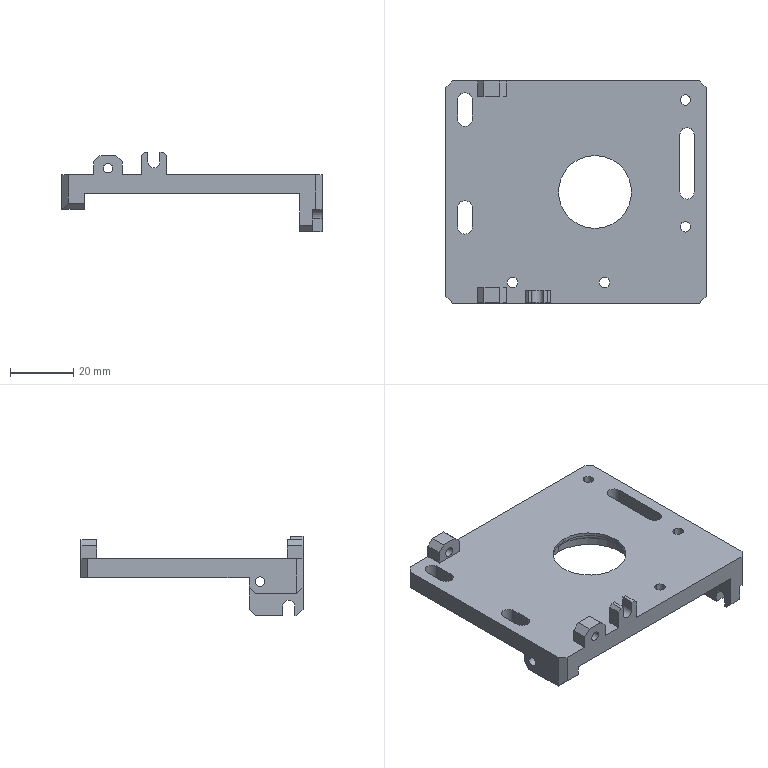NC program | NX | posted with a generic post | part box 82 x 70 x 25 mm
Lines 1 to 1705 of 7981:
N10 G17 G21 G94 G90
(FLOOR_WALL , TOOL : D20R0.8)
N12 T01 M6
N14 G54
N16 G17 G0 G90 X-56. Y36.999 S7500 M3
N18 G43 Z30. H1
N20 Z3.
N22 G94 G1 Z0. F1350.
N24 X-53.
N26 X53.
N28 Y27.479
N30 X-53.
N32 Y17.959
N34 X53.
N36 Y8.439
N38 X-53.
N40 Y-1.08
N42 X53.
N44 Y-10.6
N46 X-53.
N48 Y-20.12
N50 X53.
N52 Y-29.64
N54 X-53.
N56 X-56.
N58 Z3.
N60 G0 Z30.
N62 M5
(ZLEVEL_PROFILE_1 , TOOL : D6)
N64 T06 M6
N66 G54
N68 G17 G0 G90 X-34.289 Y38.1 S9500 M3
N70 G43 Z30. H6
N72 Z1.5
N74 G94 G1 X0. Z-0.297 F1000.
N76 X39. F3000.
N78 G2 X41.192 Y37.192 R3.1
N80 G1 X43.192 Y35.192
N82 G2 X44.1 Y33. R3.1
N84 G1 Y-33.
N86 G2 X43.192 Y-35.192 R3.1
N88 G1 X41.192 Y-37.192
N90 G2 X39. Y-38.1 R3.1
N92 G1 X-39.
N94 G2 X-41.192 Y-37.192 R3.1
N96 G1 X-43.192 Y-35.192
N98 G2 X-44.1 Y-33. R3.1
N100 G1 Y33.
N102 G2 X-43.192 Y35.192 R3.1
N104 G1 X-41.192 Y37.192
N106 G2 X-39. Y38.1 R3.1
N108 G1 X0.
N110 X17.016 Z-0.594
N112 X39.
N114 G2 X41.192 Y37.192 R3.1
N116 G1 X43.192 Y35.192
N118 G2 X44.1 Y33. R3.1
N120 G1 Y-33.
N122 G2 X43.192 Y-35.192 R3.1
N124 G1 X41.192 Y-37.192
N126 G2 X39. Y-38.1 R3.1
N128 G1 X-39.
N130 G2 X-41.192 Y-37.192 R3.1
N132 G1 X-43.192 Y-35.192
N134 G2 X-44.1 Y-33. R3.1
N136 G1 Y33.
N138 G2 X-43.192 Y35.192 R3.1
N140 G1 X-41.192 Y37.192
N142 G2 X-39. Y38.1 R3.1
N144 G1 X0.
N146 X17.016 Z-0.891
N148 X39.
N150 G2 X41.192 Y37.192 R3.1
N152 G1 X43.192 Y35.192
N154 G2 X44.1 Y33. R3.1
N156 G1 Y-33.
N158 G2 X43.192 Y-35.192 R3.1
N160 G1 X41.192 Y-37.192
N162 G2 X39. Y-38.1 R3.1
N164 G1 X-39.
N166 G2 X-41.192 Y-37.192 R3.1
N168 G1 X-43.192 Y-35.192
N170 G2 X-44.1 Y-33. R3.1
N172 G1 Y33.
N174 G2 X-43.192 Y35.192 R3.1
N176 G1 X-41.192 Y37.192
N178 G2 X-39. Y38.1 R3.1
N180 G1 X0.
N182 X17.016 Z-1.188
N184 X39.
N186 G2 X41.192 Y37.192 R3.1
N188 G1 X43.192 Y35.192
N190 G2 X44.1 Y33. R3.1
N192 G1 Y-33.
N194 G2 X43.192 Y-35.192 R3.1
N196 G1 X41.192 Y-37.192
N198 G2 X39. Y-38.1 R3.1
N200 G1 X-39.
N202 G2 X-41.192 Y-37.192 R3.1
N204 G1 X-43.192 Y-35.192
N206 G2 X-44.1 Y-33. R3.1
N208 G1 Y33.
N210 G2 X-43.192 Y35.192 R3.1
N212 G1 X-41.192 Y37.192
N214 G2 X-39. Y38.1 R3.1
N216 G1 X0.
N218 X17.016 Z-1.485
N220 X39.
N222 G2 X41.192 Y37.192 R3.1
N224 G1 X43.192 Y35.192
N226 G2 X44.1 Y33. R3.1
N228 G1 Y-33.
N230 G2 X43.192 Y-35.192 R3.1
N232 G1 X41.192 Y-37.192
N234 G2 X39. Y-38.1 R3.1
N236 G1 X-39.
N238 G2 X-41.192 Y-37.192 R3.1
N240 G1 X-43.192 Y-35.192
N242 G2 X-44.1 Y-33. R3.1
N244 G1 Y33.
N246 G2 X-43.192 Y35.192 R3.1
N248 G1 X-41.192 Y37.192
N250 G2 X-39. Y38.1 R3.1
N252 G1 X0.
N254 X17.016 Z-1.782
N256 X39.
N258 G2 X41.192 Y37.192 R3.1
N260 G1 X43.192 Y35.192
N262 G2 X44.1 Y33. R3.1
N264 G1 Y-33.
N266 G2 X43.192 Y-35.192 R3.1
N268 G1 X41.192 Y-37.192
N270 G2 X39. Y-38.1 R3.1
N272 G1 X-39.
N274 G2 X-41.192 Y-37.192 R3.1
N276 G1 X-43.192 Y-35.192
N278 G2 X-44.1 Y-33. R3.1
N280 G1 Y33.
N282 G2 X-43.192 Y35.192 R3.1
N284 G1 X-41.192 Y37.192
N286 G2 X-39. Y38.1 R3.1
N288 G1 X0.
N290 X17.016 Z-2.079
N292 X39.
N294 G2 X41.192 Y37.192 R3.1
N296 G1 X43.192 Y35.192
N298 G2 X44.1 Y33. R3.1
N300 G1 Y-33.
N302 G2 X43.192 Y-35.192 R3.1
N304 G1 X41.192 Y-37.192
N306 G2 X39. Y-38.1 R3.1
N308 G1 X-39.
N310 G2 X-41.192 Y-37.192 R3.1
N312 G1 X-43.192 Y-35.192
N314 G2 X-44.1 Y-33. R3.1
N316 G1 Y33.
N318 G2 X-43.192 Y35.192 R3.1
N320 G1 X-41.192 Y37.192
N322 G2 X-39. Y38.1 R3.1
N324 G1 X0.
N326 X17.016 Z-2.376
N328 X39.
N330 G2 X41.192 Y37.192 R3.1
N332 G1 X43.192 Y35.192
N334 G2 X44.1 Y33. R3.1
N336 G1 Y-33.
N338 G2 X43.192 Y-35.192 R3.1
N340 G1 X41.192 Y-37.192
N342 G2 X39. Y-38.1 R3.1
N344 G1 X-39.
N346 G2 X-41.192 Y-37.192 R3.1
N348 G1 X-43.192 Y-35.192
N350 G2 X-44.1 Y-33. R3.1
N352 G1 Y33.
N354 G2 X-43.192 Y35.192 R3.1
N356 G1 X-41.192 Y37.192
N358 G2 X-39. Y38.1 R3.1
N360 G1 X0.
N362 X17.016 Z-2.673
N364 X39.
N366 G2 X41.192 Y37.192 R3.1
N368 G1 X43.192 Y35.192
N370 G2 X44.1 Y33. R3.1
N372 G1 Y-33.
N374 G2 X43.192 Y-35.192 R3.1
N376 G1 X41.192 Y-37.192
N378 G2 X39. Y-38.1 R3.1
N380 G1 X-39.
N382 G2 X-41.192 Y-37.192 R3.1
N384 G1 X-43.192 Y-35.192
N386 G2 X-44.1 Y-33. R3.1
N388 G1 Y33.
N390 G2 X-43.192 Y35.192 R3.1
N392 G1 X-41.192 Y37.192
N394 G2 X-39. Y38.1 R3.1
N396 G1 X0.
N398 X17.016 Z-2.97
N400 X39.
N402 G2 X41.192 Y37.192 R3.1
N404 G1 X43.192 Y35.192
N406 G2 X44.1 Y33. R3.1
N408 G1 Y-33.
N410 G2 X43.192 Y-35.192 R3.1
N412 G1 X41.192 Y-37.192
N414 G2 X39. Y-38.1 R3.1
N416 G1 X-39.
N418 G2 X-41.192 Y-37.192 R3.1
N420 G1 X-43.192 Y-35.192
N422 G2 X-44.1 Y-33. R3.1
N424 G1 Y33.
N426 G2 X-43.192 Y35.192 R3.1
N428 G1 X-41.192 Y37.192
N430 G2 X-39. Y38.1 R3.1
N432 G1 X0.
N434 X17.016 Z-3.267
N436 X39.
N438 G2 X41.192 Y37.192 R3.1
N440 G1 X43.192 Y35.192
N442 G2 X44.1 Y33. R3.1
N444 G1 Y-33.
N446 G2 X43.192 Y-35.192 R3.1
N448 G1 X41.192 Y-37.192
N450 G2 X39. Y-38.1 R3.1
N452 G1 X-39.
N454 G2 X-41.192 Y-37.192 R3.1
N456 G1 X-43.192 Y-35.192
N458 G2 X-44.1 Y-33. R3.1
N460 G1 Y33.
N462 G2 X-43.192 Y35.192 R3.1
N464 G1 X-41.192 Y37.192
N466 G2 X-39. Y38.1 R3.1
N468 G1 X0.
N470 X17.016 Z-3.564
N472 X39.
N474 G2 X41.192 Y37.192 R3.1
N476 G1 X43.192 Y35.192
N478 G2 X44.1 Y33. R3.1
N480 G1 Y-33.
N482 G2 X43.192 Y-35.192 R3.1
N484 G1 X41.192 Y-37.192
N486 G2 X39. Y-38.1 R3.1
N488 G1 X-39.
N490 G2 X-41.192 Y-37.192 R3.1
N492 G1 X-43.192 Y-35.192
N494 G2 X-44.1 Y-33. R3.1
N496 G1 Y33.
N498 G2 X-43.192 Y35.192 R3.1
N500 G1 X-41.192 Y37.192
N502 G2 X-39. Y38.1 R3.1
N504 G1 X0.
N506 X17.016 Z-3.861
N508 X39.
N510 G2 X41.192 Y37.192 R3.1
N512 G1 X43.192 Y35.192
N514 G2 X44.1 Y33. R3.1
N516 G1 Y-33.
N518 G2 X43.192 Y-35.192 R3.1
N520 G1 X41.192 Y-37.192
N522 G2 X39. Y-38.1 R3.1
N524 G1 X-39.
N526 G2 X-41.192 Y-37.192 R3.1
N528 G1 X-43.192 Y-35.192
N530 G2 X-44.1 Y-33. R3.1
N532 G1 Y33.
N534 G2 X-43.192 Y35.192 R3.1
N536 G1 X-41.192 Y37.192
N538 G2 X-39. Y38.1 R3.1
N540 G1 X0.
N542 X17.016 Z-4.158
N544 X39.
N546 G2 X41.192 Y37.192 R3.1
N548 G1 X43.192 Y35.192
N550 G2 X44.1 Y33. R3.1
N552 G1 Y-33.
N554 G2 X43.192 Y-35.192 R3.1
N556 G1 X41.192 Y-37.192
N558 G2 X39. Y-38.1 R3.1
N560 G1 X-39.
N562 G2 X-41.192 Y-37.192 R3.1
N564 G1 X-43.192 Y-35.192
N566 G2 X-44.1 Y-33. R3.1
N568 G1 Y33.
N570 G2 X-43.192 Y35.192 R3.1
N572 G1 X-41.192 Y37.192
N574 G2 X-39. Y38.1 R3.1
N576 G1 X0.
N578 X17.016 Z-4.455
N580 X39.
N582 G2 X41.192 Y37.192 R3.1
N584 G1 X43.192 Y35.192
N586 G2 X44.1 Y33. R3.1
N588 G1 Y-33.
N590 G2 X43.192 Y-35.192 R3.1
N592 G1 X41.192 Y-37.192
N594 G2 X39. Y-38.1 R3.1
N596 G1 X-39.
N598 G2 X-41.192 Y-37.192 R3.1
N600 G1 X-43.192 Y-35.192
N602 G2 X-44.1 Y-33. R3.1
N604 G1 Y33.
N606 G2 X-43.192 Y35.192 R3.1
N608 G1 X-41.192 Y37.192
N610 G2 X-39. Y38.1 R3.1
N612 G1 X0.
N614 X17.016 Z-4.752
N616 X39.
N618 G2 X41.192 Y37.192 R3.1
N620 G1 X43.192 Y35.192
N622 G2 X44.1 Y33. R3.1
N624 G1 Y-33.
N626 G2 X43.192 Y-35.192 R3.1
N628 G1 X41.192 Y-37.192
N630 G2 X39. Y-38.1 R3.1
N632 G1 X-39.
N634 G2 X-41.192 Y-37.192 R3.1
N636 G1 X-43.192 Y-35.192
N638 G2 X-44.1 Y-33. R3.1
N640 G1 Y33.
N642 G2 X-43.192 Y35.192 R3.1
N644 G1 X-41.192 Y37.192
N646 G2 X-39. Y38.1 R3.1
N648 G1 X0.
N650 X17.016 Z-5.049
N652 X39.
N654 G2 X41.192 Y37.192 R3.1
N656 G1 X43.192 Y35.192
N658 G2 X44.1 Y33. R3.1
N660 G1 Y-33.
N662 G2 X43.192 Y-35.192 R3.1
N664 G1 X41.192 Y-37.192
N666 G2 X39. Y-38.1 R3.1
N668 G1 X-39.
N670 G2 X-41.192 Y-37.192 R3.1
N672 G1 X-43.192 Y-35.192
N674 G2 X-44.1 Y-33. R3.1
N676 G1 Y33.
N678 G2 X-43.192 Y35.192 R3.1
N680 G1 X-41.192 Y37.192
N682 G2 X-39. Y38.1 R3.1
N684 G1 X0.
N686 X17.016 Z-5.346
N688 X39.
N690 G2 X41.192 Y37.192 R3.1
N692 G1 X43.192 Y35.192
N694 G2 X44.1 Y33. R3.1
N696 G1 Y-33.
N698 G2 X43.192 Y-35.192 R3.1
N700 G1 X41.192 Y-37.192
N702 G2 X39. Y-38.1 R3.1
N704 G1 X-39.
N706 G2 X-41.192 Y-37.192 R3.1
N708 G1 X-43.192 Y-35.192
N710 G2 X-44.1 Y-33. R3.1
N712 G1 Y33.
N714 G2 X-43.192 Y35.192 R3.1
N716 G1 X-41.192 Y37.192
N718 G2 X-39. Y38.1 R3.1
N720 G1 X0.
N722 X17.016 Z-5.643
N724 X39.
N726 G2 X41.192 Y37.192 R3.1
N728 G1 X43.192 Y35.192
N730 G2 X44.1 Y33. R3.1
N732 G1 Y-33.
N734 G2 X43.192 Y-35.192 R3.1
N736 G1 X41.192 Y-37.192
N738 G2 X39. Y-38.1 R3.1
N740 G1 X-39.
N742 G2 X-41.192 Y-37.192 R3.1
N744 G1 X-43.192 Y-35.192
N746 G2 X-44.1 Y-33. R3.1
N748 G1 Y33.
N750 G2 X-43.192 Y35.192 R3.1
N752 G1 X-41.192 Y37.192
N754 G2 X-39. Y38.1 R3.1
N756 G1 X0.
N758 X17.016 Z-5.94
N760 X39.
N762 G2 X41.192 Y37.192 R3.1
N764 G1 X43.192 Y35.192
N766 G2 X44.1 Y33. R3.1
N768 G1 Y-33.
N770 G2 X43.192 Y-35.192 R3.1
N772 G1 X41.192 Y-37.192
N774 G2 X39. Y-38.1 R3.1
N776 G1 X-39.
N778 G2 X-41.192 Y-37.192 R3.1
N780 G1 X-43.192 Y-35.192
N782 G2 X-44.1 Y-33. R3.1
N784 G1 Y33.
N786 G2 X-43.192 Y35.192 R3.1
N788 G1 X-41.192 Y37.192
N790 G2 X-39. Y38.1 R3.1
N792 G1 X0.
N794 X17.016 Z-6.238
N796 X39.
N798 G2 X41.192 Y37.192 R3.1
N800 G1 X43.192 Y35.192
N802 G2 X44.1 Y33. R3.1
N804 G1 Y-33.
N806 G2 X43.192 Y-35.192 R3.1
N808 G1 X41.192 Y-37.192
N810 G2 X39. Y-38.1 R3.1
N812 G1 X-39.
N814 G2 X-41.192 Y-37.192 R3.1
N816 G1 X-43.192 Y-35.192
N818 G2 X-44.1 Y-33. R3.1
N820 G1 Y33.
N822 G2 X-43.192 Y35.192 R3.1
N824 G1 X-41.192 Y37.192
N826 G2 X-39. Y38.1 R3.1
N828 G1 X0.
N830 X17.016 Z-6.535
N832 X39.
N834 G2 X41.192 Y37.192 R3.1
N836 G1 X43.192 Y35.192
N838 G2 X44.1 Y33. R3.1
N840 G1 Y-33.
N842 G2 X43.192 Y-35.192 R3.1
N844 G1 X41.192 Y-37.192
N846 G2 X39. Y-38.1 R3.1
N848 G1 X-39.
N850 G2 X-41.192 Y-37.192 R3.1
N852 G1 X-43.192 Y-35.192
N854 G2 X-44.1 Y-33. R3.1
N856 G1 Y33.
N858 G2 X-43.192 Y35.192 R3.1
N860 G1 X-41.192 Y37.192
N862 G2 X-39. Y38.1 R3.1
N864 G1 X0.
N866 X17.016 Z-6.832
N868 X39.
N870 G2 X41.192 Y37.192 R3.1
N872 G1 X43.192 Y35.192
N874 G2 X44.1 Y33. R3.1
N876 G1 Y-33.
N878 G2 X43.192 Y-35.192 R3.1
N880 G1 X41.192 Y-37.192
N882 G2 X39. Y-38.1 R3.1
N884 G1 X-39.
N886 G2 X-41.192 Y-37.192 R3.1
N888 G1 X-43.192 Y-35.192
N890 G2 X-44.1 Y-33. R3.1
N892 G1 Y33.
N894 G2 X-43.192 Y35.192 R3.1
N896 G1 X-41.192 Y37.192
N898 G2 X-39. Y38.1 R3.1
N900 G1 X0.
N902 X17.016 Z-7.129
N904 X39.
N906 G2 X41.192 Y37.192 R3.1
N908 G1 X43.192 Y35.192
N910 G2 X44.1 Y33. R3.1
N912 G1 Y-33.
N914 G2 X43.192 Y-35.192 R3.1
N916 G1 X41.192 Y-37.192
N918 G2 X39. Y-38.1 R3.1
N920 G1 X-39.
N922 G2 X-41.192 Y-37.192 R3.1
N924 G1 X-43.192 Y-35.192
N926 G2 X-44.1 Y-33. R3.1
N928 G1 Y33.
N930 G2 X-43.192 Y35.192 R3.1
N932 G1 X-41.192 Y37.192
N934 G2 X-39. Y38.1 R3.1
N936 G1 X0.
N938 X17.016 Z-7.426
N940 X39.
N942 G2 X41.192 Y37.192 R3.1
N944 G1 X43.192 Y35.192
N946 G2 X44.1 Y33. R3.1
N948 G1 Y-33.
N950 G2 X43.192 Y-35.192 R3.1
N952 G1 X41.192 Y-37.192
N954 G2 X39. Y-38.1 R3.1
N956 G1 X-39.
N958 G2 X-41.192 Y-37.192 R3.1
N960 G1 X-43.192 Y-35.192
N962 G2 X-44.1 Y-33. R3.1
N964 G1 Y33.
N966 G2 X-43.192 Y35.192 R3.1
N968 G1 X-41.192 Y37.192
N970 G2 X-39. Y38.1 R3.1
N972 G1 X0.
N974 X17.016 Z-7.723
N976 X39.
N978 G2 X41.192 Y37.192 R3.1
N980 G1 X43.192 Y35.192
N982 G2 X44.1 Y33. R3.1
N984 G1 Y-33.
N986 G2 X43.192 Y-35.192 R3.1
N988 G1 X41.192 Y-37.192
N990 G2 X39. Y-38.1 R3.1
N992 G1 X-39.
N994 G2 X-41.192 Y-37.192 R3.1
N996 G1 X-43.192 Y-35.192
N998 G2 X-44.1 Y-33. R3.1
N1000 G1 Y33.
N1002 G2 X-43.192 Y35.192 R3.1
N1004 G1 X-41.192 Y37.192
N1006 G2 X-39. Y38.1 R3.1
N1008 G1 X0.
N1010 X17.016 Z-8.02
N1012 X39.
N1014 G2 X41.192 Y37.192 R3.1
N1016 G1 X43.192 Y35.192
N1018 G2 X44.1 Y33. R3.1
N1020 G1 Y-33.
N1022 G2 X43.192 Y-35.192 R3.1
N1024 G1 X41.192 Y-37.192
N1026 G2 X39. Y-38.1 R3.1
N1028 G1 X-39.
N1030 G2 X-41.192 Y-37.192 R3.1
N1032 G1 X-43.192 Y-35.192
N1034 G2 X-44.1 Y-33. R3.1
N1036 G1 Y33.
N1038 G2 X-43.192 Y35.192 R3.1
N1040 G1 X-41.192 Y37.192
N1042 G2 X-39. Y38.1 R3.1
N1044 G1 X0.
N1046 X17.016 Z-8.317
N1048 X39.
N1050 G2 X41.192 Y37.192 R3.1
N1052 G1 X43.192 Y35.192
N1054 G2 X44.1 Y33. R3.1
N1056 G1 Y-33.
N1058 G2 X43.192 Y-35.192 R3.1
N1060 G1 X41.192 Y-37.192
N1062 G2 X39. Y-38.1 R3.1
N1064 G1 X-39.
N1066 G2 X-41.192 Y-37.192 R3.1
N1068 G1 X-43.192 Y-35.192
N1070 G2 X-44.1 Y-33. R3.1
N1072 G1 Y33.
N1074 G2 X-43.192 Y35.192 R3.1
N1076 G1 X-41.192 Y37.192
N1078 G2 X-39. Y38.1 R3.1
N1080 G1 X0.
N1082 X17.016 Z-8.614
N1084 X39.
N1086 G2 X41.192 Y37.192 R3.1
N1088 G1 X43.192 Y35.192
N1090 G2 X44.1 Y33. R3.1
N1092 G1 Y-33.
N1094 G2 X43.192 Y-35.192 R3.1
N1096 G1 X41.192 Y-37.192
N1098 G2 X39. Y-38.1 R3.1
N1100 G1 X-39.
N1102 G2 X-41.192 Y-37.192 R3.1
N1104 G1 X-43.192 Y-35.192
N1106 G2 X-44.1 Y-33. R3.1
N1108 G1 Y33.
N1110 G2 X-43.192 Y35.192 R3.1
N1112 G1 X-41.192 Y37.192
N1114 G2 X-39. Y38.1 R3.1
N1116 G1 X0.
N1118 X17.016 Z-8.911
N1120 X39.
N1122 G2 X41.192 Y37.192 R3.1
N1124 G1 X43.192 Y35.192
N1126 G2 X44.1 Y33. R3.1
N1128 G1 Y-33.
N1130 G2 X43.192 Y-35.192 R3.1
N1132 G1 X41.192 Y-37.192
N1134 G2 X39. Y-38.1 R3.1
N1136 G1 X-39.
N1138 G2 X-41.192 Y-37.192 R3.1
N1140 G1 X-43.192 Y-35.192
N1142 G2 X-44.1 Y-33. R3.1
N1144 G1 Y33.
N1146 G2 X-43.192 Y35.192 R3.1
N1148 G1 X-41.192 Y37.192
N1150 G2 X-39. Y38.1 R3.1
N1152 G1 X0.
N1154 X17.016 Z-9.208
N1156 X39.
N1158 G2 X41.192 Y37.192 R3.1
N1160 G1 X43.192 Y35.192
N1162 G2 X44.1 Y33. R3.1
N1164 G1 Y-33.
N1166 G2 X43.192 Y-35.192 R3.1
N1168 G1 X41.192 Y-37.192
N1170 G2 X39. Y-38.1 R3.1
N1172 G1 X-39.
N1174 G2 X-41.192 Y-37.192 R3.1
N1176 G1 X-43.192 Y-35.192
N1178 G2 X-44.1 Y-33. R3.1
N1180 G1 Y33.
N1182 G2 X-43.192 Y35.192 R3.1
N1184 G1 X-41.192 Y37.192
N1186 G2 X-39. Y38.1 R3.1
N1188 G1 X0.
N1190 X17.016 Z-9.505
N1192 X39.
N1194 G2 X41.192 Y37.192 R3.1
N1196 G1 X43.192 Y35.192
N1198 G2 X44.1 Y33. R3.1
N1200 G1 Y-33.
N1202 G2 X43.192 Y-35.192 R3.1
N1204 G1 X41.192 Y-37.192
N1206 G2 X39. Y-38.1 R3.1
N1208 G1 X-39.
N1210 G2 X-41.192 Y-37.192 R3.1
N1212 G1 X-43.192 Y-35.192
N1214 G2 X-44.1 Y-33. R3.1
N1216 G1 Y33.
N1218 G2 X-43.192 Y35.192 R3.1
N1220 G1 X-41.192 Y37.192
N1222 G2 X-39. Y38.1 R3.1
N1224 G1 X0.
N1226 X17.016 Z-9.802
N1228 X39.
N1230 G2 X41.192 Y37.192 R3.1
N1232 G1 X43.192 Y35.192
N1234 G2 X44.1 Y33. R3.1
N1236 G1 Y-33.
N1238 G2 X43.192 Y-35.192 R3.1
N1240 G1 X41.192 Y-37.192
N1242 G2 X39. Y-38.1 R3.1
N1244 G1 X-39.
N1246 G2 X-41.192 Y-37.192 R3.1
N1248 G1 X-43.192 Y-35.192
N1250 G2 X-44.1 Y-33. R3.1
N1252 G1 Y33.
N1254 G2 X-43.192 Y35.192 R3.1
N1256 G1 X-41.192 Y37.192
N1258 G2 X-39. Y38.1 R3.1
N1260 G1 X0.
N1262 X17.016 Z-10.099
N1264 X39.
N1266 G2 X41.192 Y37.192 R3.1
N1268 G1 X43.192 Y35.192
N1270 G2 X44.1 Y33. R3.1
N1272 G1 Y-33.
N1274 G2 X43.192 Y-35.192 R3.1
N1276 G1 X41.192 Y-37.192
N1278 G2 X39. Y-38.1 R3.1
N1280 G1 X-39.
N1282 G2 X-41.192 Y-37.192 R3.1
N1284 G1 X-43.192 Y-35.192
N1286 G2 X-44.1 Y-33. R3.1
N1288 G1 Y33.
N1290 G2 X-43.192 Y35.192 R3.1
N1292 G1 X-41.192 Y37.192
N1294 G2 X-39. Y38.1 R3.1
N1296 G1 X0.
N1298 X17.016 Z-10.396
N1300 X39.
N1302 G2 X41.192 Y37.192 R3.1
N1304 G1 X43.192 Y35.192
N1306 G2 X44.1 Y33. R3.1
N1308 G1 Y-33.
N1310 G2 X43.192 Y-35.192 R3.1
N1312 G1 X41.192 Y-37.192
N1314 G2 X39. Y-38.1 R3.1
N1316 G1 X-39.
N1318 G2 X-41.192 Y-37.192 R3.1
N1320 G1 X-43.192 Y-35.192
N1322 G2 X-44.1 Y-33. R3.1
N1324 G1 Y33.
N1326 G2 X-43.192 Y35.192 R3.1
N1328 G1 X-41.192 Y37.192
N1330 G2 X-39. Y38.1 R3.1
N1332 G1 X0.
N1334 X17.016 Z-10.693
N1336 X39.
N1338 G2 X41.192 Y37.192 R3.1
N1340 G1 X43.192 Y35.192
N1342 G2 X44.1 Y33. R3.1
N1344 G1 Y-33.
N1346 G2 X43.192 Y-35.192 R3.1
N1348 G1 X41.192 Y-37.192
N1350 G2 X39. Y-38.1 R3.1
N1352 G1 X-39.
N1354 G2 X-41.192 Y-37.192 R3.1
N1356 G1 X-43.192 Y-35.192
N1358 G2 X-44.1 Y-33. R3.1
N1360 G1 Y33.
N1362 G2 X-43.192 Y35.192 R3.1
N1364 G1 X-41.192 Y37.192
N1366 G2 X-39. Y38.1 R3.1
N1368 G1 X0.
N1370 X17.016 Z-10.99
N1372 X39.
N1374 G2 X41.192 Y37.192 R3.1
N1376 G1 X43.192 Y35.192
N1378 G2 X44.1 Y33. R3.1
N1380 G1 Y-33.
N1382 G2 X43.192 Y-35.192 R3.1
N1384 G1 X41.192 Y-37.192
N1386 G2 X39. Y-38.1 R3.1
N1388 G1 X-39.
N1390 G2 X-41.192 Y-37.192 R3.1
N1392 G1 X-43.192 Y-35.192
N1394 G2 X-44.1 Y-33. R3.1
N1396 G1 Y33.
N1398 G2 X-43.192 Y35.192 R3.1
N1400 G1 X-41.192 Y37.192
N1402 G2 X-39. Y38.1 R3.1
N1404 G1 X0.
N1406 X17.016 Z-11.287
N1408 X39.
N1410 G2 X41.192 Y37.192 R3.1
N1412 G1 X43.192 Y35.192
N1414 G2 X44.1 Y33. R3.1
N1416 G1 Y-33.
N1418 G2 X43.192 Y-35.192 R3.1
N1420 G1 X41.192 Y-37.192
N1422 G2 X39. Y-38.1 R3.1
N1424 G1 X-39.
N1426 G2 X-41.192 Y-37.192 R3.1
N1428 G1 X-43.192 Y-35.192
N1430 G2 X-44.1 Y-33. R3.1
N1432 G1 Y33.
N1434 G2 X-43.192 Y35.192 R3.1
N1436 G1 X-41.192 Y37.192
N1438 G2 X-39. Y38.1 R3.1
N1440 G1 X0.
N1442 X17.016 Z-11.584
N1444 X39.
N1446 G2 X41.192 Y37.192 R3.1
N1448 G1 X43.192 Y35.192
N1450 G2 X44.1 Y33. R3.1
N1452 G1 Y-33.
N1454 G2 X43.192 Y-35.192 R3.1
N1456 G1 X41.192 Y-37.192
N1458 G2 X39. Y-38.1 R3.1
N1460 G1 X-39.
N1462 G2 X-41.192 Y-37.192 R3.1
N1464 G1 X-43.192 Y-35.192
N1466 G2 X-44.1 Y-33. R3.1
N1468 G1 Y33.
N1470 G2 X-43.192 Y35.192 R3.1
N1472 G1 X-41.192 Y37.192
N1474 G2 X-39. Y38.1 R3.1
N1476 G1 X0.
N1478 X17.016 Z-11.881
N1480 X39.
N1482 G2 X41.192 Y37.192 R3.1
N1484 G1 X43.192 Y35.192
N1486 G2 X44.1 Y33. R3.1
N1488 G1 Y-33.
N1490 G2 X43.192 Y-35.192 R3.1
N1492 G1 X41.192 Y-37.192
N1494 G2 X39. Y-38.1 R3.1
N1496 G1 X-39.
N1498 G2 X-41.192 Y-37.192 R3.1
N1500 G1 X-43.192 Y-35.192
N1502 G2 X-44.1 Y-33. R3.1
N1504 G1 Y33.
N1506 G2 X-43.192 Y35.192 R3.1
N1508 G1 X-41.192 Y37.192
N1510 G2 X-39. Y38.1 R3.1
N1512 G1 X0.
N1514 X17.016 Z-12.178
N1516 X39.
N1518 G2 X41.192 Y37.192 R3.1
N1520 G1 X43.192 Y35.192
N1522 G2 X44.1 Y33. R3.1
N1524 G1 Y-33.
N1526 G2 X43.192 Y-35.192 R3.1
N1528 G1 X41.192 Y-37.192
N1530 G2 X39. Y-38.1 R3.1
N1532 G1 X-39.
N1534 G2 X-41.192 Y-37.192 R3.1
N1536 G1 X-43.192 Y-35.192
N1538 G2 X-44.1 Y-33. R3.1
N1540 G1 Y33.
N1542 G2 X-43.192 Y35.192 R3.1
N1544 G1 X-41.192 Y37.192
N1546 G2 X-39. Y38.1 R3.1
N1548 G1 X0.
N1550 X17.016 Z-12.475
N1552 X39.
N1554 G2 X41.192 Y37.192 R3.1
N1556 G1 X43.192 Y35.192
N1558 G2 X44.1 Y33. R3.1
N1560 G1 Y-33.
N1562 G2 X43.192 Y-35.192 R3.1
N1564 G1 X41.192 Y-37.192
N1566 G2 X39. Y-38.1 R3.1
N1568 G1 X-39.
N1570 G2 X-41.192 Y-37.192 R3.1
N1572 G1 X-43.192 Y-35.192
N1574 G2 X-44.1 Y-33. R3.1
N1576 G1 Y33.
N1578 G2 X-43.192 Y35.192 R3.1
N1580 G1 X-41.192 Y37.192
N1582 G2 X-39. Y38.1 R3.1
N1584 G1 X0.
N1586 X17.016 Z-12.772
N1588 X39.
N1590 G2 X41.192 Y37.192 R3.1
N1592 G1 X43.192 Y35.192
N1594 G2 X44.1 Y33. R3.1
N1596 G1 Y-33.
N1598 G2 X43.192 Y-35.192 R3.1
N1600 G1 X41.192 Y-37.192
N1602 G2 X39. Y-38.1 R3.1
N1604 G1 X-39.
N1606 G2 X-41.192 Y-37.192 R3.1
N1608 G1 X-43.192 Y-35.192
N1610 G2 X-44.1 Y-33. R3.1
N1612 G1 Y33.
N1614 G2 X-43.192 Y35.192 R3.1
N1616 G1 X-41.192 Y37.192
N1618 G2 X-39. Y38.1 R3.1
N1620 G1 X0.
N1622 X17.016 Z-13.069
N1624 X39.
N1626 G2 X41.192 Y37.192 R3.1
N1628 G1 X43.192 Y35.192
N1630 G2 X44.1 Y33. R3.1
N1632 G1 Y-33.
N1634 G2 X43.192 Y-35.192 R3.1
N1636 G1 X41.192 Y-37.192
N1638 G2 X39. Y-38.1 R3.1
N1640 G1 X-39.
N1642 G2 X-41.192 Y-37.192 R3.1
N1644 G1 X-43.192 Y-35.192
N1646 G2 X-44.1 Y-33. R3.1
N1648 G1 Y33.
N1650 G2 X-43.192 Y35.192 R3.1
N1652 G1 X-41.192 Y37.192
N1654 G2 X-39. Y38.1 R3.1
N1656 G1 X0.
N1658 X17.016 Z-13.366
N1660 X39.
N1662 G2 X41.192 Y37.192 R3.1
N1664 G1 X43.192 Y35.192
N1666 G2 X44.1 Y33. R3.1
N1668 G1 Y-33.
N1670 G2 X43.192 Y-35.192 R3.1
N1672 G1 X41.192 Y-37.192
N1674 G2 X39. Y-38.1 R3.1
N1676 G1 X-39.
N1678 G2 X-41.192 Y-37.192 R3.1
N1680 G1 X-43.192 Y-35.192
N1682 G2 X-44.1 Y-33. R3.1
N1684 G1 Y33.
N1686 G2 X-43.192 Y35.192 R3.1
N1688 G1 X-41.192 Y37.192
N1690 G2 X-39. Y38.1 R3.1
N1692 G1 X0.
N1694 X17.016 Z-13.663
N1696 X39.
N1698 G2 X41.192 Y37.192 R3.1
N1700 G1 X43.192 Y35.192
N1702 G2 X44.1 Y33. R3.1
N1704 G1 Y-33.
N1706 G2 X43.192 Y-35.192 R3.1
N1708 G1 X41.192 Y-37.192
N1710 G2 X39. Y-38.1 R3.1
N1712 G1 X-39.
N1714 G2 X-41.192 Y-37.192 R3.1
N1716 G1 X-43.192 Y-35.192
N1718 G2 X-44.1 Y-33. R3.1
N1720 G1 Y33.
N1722 G2 X-43.192 Y35.192 R3.1
N1724 G1 X-41.192 Y37.192
N1726 G2 X-39. Y38.1 R3.1
N1728 G1 X0.
N1730 X17.016 Z-13.96
N1732 X39.
N1734 G2 X41.192 Y37.192 R3.1
N1736 G1 X43.192 Y35.192
N1738 G2 X44.1 Y33. R3.1
N1740 G1 Y-33.
N1742 G2 X43.192 Y-35.192 R3.1
N1744 G1 X41.192 Y-37.192
N1746 G2 X39. Y-38.1 R3.1
N1748 G1 X-39.
N1750 G2 X-41.192 Y-37.192 R3.1
N1752 G1 X-43.192 Y-35.192
N1754 G2 X-44.1 Y-33. R3.1
N1756 G1 Y33.
N1758 G2 X-43.192 Y35.192 R3.1
N1760 G1 X-41.192 Y37.192
N1762 G2 X-39. Y38.1 R3.1
N1764 G1 X0.
N1766 X17.016 Z-14.257
N1768 X39.
N1770 G2 X41.192 Y37.192 R3.1
N1772 G1 X43.192 Y35.192
N1774 G2 X44.1 Y33. R3.1
N1776 G1 Y-33.
N1778 G2 X43.192 Y-35.192 R3.1
N1780 G1 X41.192 Y-37.192
N1782 G2 X39. Y-38.1 R3.1
N1784 G1 X-39.
N1786 G2 X-41.192 Y-37.192 R3.1
N1788 G1 X-43.192 Y-35.192
N1790 G2 X-44.1 Y-33. R3.1
N1792 G1 Y33.
N1794 G2 X-43.192 Y35.192 R3.1
N1796 G1 X-41.192 Y37.192
N1798 G2 X-39. Y38.1 R3.1
N1800 G1 X0.
N1802 X17.016 Z-14.554
N1804 X39.
N1806 G2 X41.192 Y37.192 R3.1
N1808 G1 X43.192 Y35.192
N1810 G2 X44.1 Y33. R3.1
N1812 G1 Y-33.
N1814 G2 X43.192 Y-35.192 R3.1
N1816 G1 X41.192 Y-37.192
N1818 G2 X39. Y-38.1 R3.1
N1820 G1 X-39.
N1822 G2 X-41.192 Y-37.192 R3.1
N1824 G1 X-43.192 Y-35.192
N1826 G2 X-44.1 Y-33. R3.1
N1828 G1 Y33.
N1830 G2 X-43.192 Y35.192 R3.1
N1832 G1 X-41.192 Y37.192
N1834 G2 X-39. Y38.1 R3.1
N1836 G1 X0.
N1838 X17.016 Z-14.851
N1840 X39.
N1842 G2 X41.192 Y37.192 R3.1
N1844 G1 X43.192 Y35.192
N1846 G2 X44.1 Y33. R3.1
N1848 G1 Y-33.
N1850 G2 X43.192 Y-35.192 R3.1
N1852 G1 X41.192 Y-37.192
N1854 G2 X39. Y-38.1 R3.1
N1856 G1 X-39.
N1858 G2 X-41.192 Y-37.192 R3.1
N1860 G1 X-43.192 Y-35.192
N1862 G2 X-44.1 Y-33. R3.1
N1864 G1 Y33.
N1866 G2 X-43.192 Y35.192 R3.1
N1868 G1 X-41.192 Y37.192
N1870 G2 X-39. Y38.1 R3.1
N1872 G1 X0.
N1874 X17.016 Z-15.148
N1876 X39.
N1878 G2 X41.192 Y37.192 R3.1
N1880 G1 X43.192 Y35.192
N1882 G2 X44.1 Y33. R3.1
N1884 G1 Y-33.
N1886 G2 X43.192 Y-35.192 R3.1
N1888 G1 X41.192 Y-37.192
N1890 G2 X39. Y-38.1 R3.1
N1892 G1 X-39.
N1894 G2 X-41.192 Y-37.192 R3.1
N1896 G1 X-43.192 Y-35.192
N1898 G2 X-44.1 Y-33. R3.1
N1900 G1 Y33.
N1902 G2 X-43.192 Y35.192 R3.1
N1904 G1 X-41.192 Y37.192
N1906 G2 X-39. Y38.1 R3.1
N1908 G1 X0.
N1910 X17.016 Z-15.445
N1912 X39.
N1914 G2 X41.192 Y37.192 R3.1
N1916 G1 X43.192 Y35.192
N1918 G2 X44.1 Y33. R3.1
N1920 G1 Y-33.
N1922 G2 X43.192 Y-35.192 R3.1
N1924 G1 X41.192 Y-37.192
N1926 G2 X39. Y-38.1 R3.1
N1928 G1 X-39.
N1930 G2 X-41.192 Y-37.192 R3.1
N1932 G1 X-43.192 Y-35.192
N1934 G2 X-44.1 Y-33. R3.1
N1936 G1 Y33.
N1938 G2 X-43.192 Y35.192 R3.1
N1940 G1 X-41.192 Y37.192
N1942 G2 X-39. Y38.1 R3.1
N1944 G1 X0.
N1946 X17.016 Z-15.742
N1948 X39.
N1950 G2 X41.192 Y37.192 R3.1
N1952 G1 X43.192 Y35.192
N1954 G2 X44.1 Y33. R3.1
N1956 G1 Y-33.
N1958 G2 X43.192 Y-35.192 R3.1
N1960 G1 X41.192 Y-37.192
N1962 G2 X39. Y-38.1 R3.1
N1964 G1 X-39.
N1966 G2 X-41.192 Y-37.192 R3.1
N1968 G1 X-43.192 Y-35.192
N1970 G2 X-44.1 Y-33. R3.1
N1972 G1 Y33.
N1974 G2 X-43.192 Y35.192 R3.1
N1976 G1 X-41.192 Y37.192
N1978 G2 X-39. Y38.1 R3.1
N1980 G1 X0.
N1982 X17.016 Z-16.039
N1984 X39.
N1986 G2 X41.192 Y37.192 R3.1
N1988 G1 X43.192 Y35.192
N1990 G2 X44.1 Y33. R3.1
N1992 G1 Y-33.
N1994 G2 X43.192 Y-35.192 R3.1
N1996 G1 X41.192 Y-37.192
N1998 G2 X39. Y-38.1 R3.1
N2000 G1 X-39.
N2002 G2 X-41.192 Y-37.192 R3.1
N2004 G1 X-43.192 Y-35.192
N2006 G2 X-44.1 Y-33. R3.1
N2008 G1 Y33.
N2010 G2 X-43.192 Y35.192 R3.1
N2012 G1 X-41.192 Y37.192
N2014 G2 X-39. Y38.1 R3.1
N2016 G1 X0.
N2018 X17.016 Z-16.336
N2020 X39.
N2022 G2 X41.192 Y37.192 R3.1
N2024 G1 X43.192 Y35.192
N2026 G2 X44.1 Y33. R3.1
N2028 G1 Y-33.
N2030 G2 X43.192 Y-35.192 R3.1
N2032 G1 X41.192 Y-37.192
N2034 G2 X39. Y-38.1 R3.1
N2036 G1 X-39.
N2038 G2 X-41.192 Y-37.192 R3.1
N2040 G1 X-43.192 Y-35.192
N2042 G2 X-44.1 Y-33. R3.1
N2044 G1 Y33.
N2046 G2 X-43.192 Y35.192 R3.1
N2048 G1 X-41.192 Y37.192
N2050 G2 X-39. Y38.1 R3.1
N2052 G1 X0.
N2054 X17.016 Z-16.633
N2056 X39.
N2058 G2 X41.192 Y37.192 R3.1
N2060 G1 X43.192 Y35.192
N2062 G2 X44.1 Y33. R3.1
N2064 G1 Y-33.
N2066 G2 X43.192 Y-35.192 R3.1
N2068 G1 X41.192 Y-37.192
N2070 G2 X39. Y-38.1 R3.1
N2072 G1 X-39.
N2074 G2 X-41.192 Y-37.192 R3.1
N2076 G1 X-43.192 Y-35.192
N2078 G2 X-44.1 Y-33. R3.1
N2080 G1 Y33.
N2082 G2 X-43.192 Y35.192 R3.1
N2084 G1 X-41.192 Y37.192
N2086 G2 X-39. Y38.1 R3.1
N2088 G1 X0.
N2090 X17.016 Z-16.93
N2092 X39.
N2094 G2 X41.192 Y37.192 R3.1
N2096 G1 X43.192 Y35.192
N2098 G2 X44.1 Y33. R3.1
N2100 G1 Y-33.
N2102 G2 X43.192 Y-35.192 R3.1
N2104 G1 X41.192 Y-37.192
N2106 G2 X39. Y-38.1 R3.1
N2108 G1 X-39.
N2110 G2 X-41.192 Y-37.192 R3.1
N2112 G1 X-43.192 Y-35.192
N2114 G2 X-44.1 Y-33. R3.1
N2116 G1 Y33.
N2118 G2 X-43.192 Y35.192 R3.1
N2120 G1 X-41.192 Y37.192
N2122 G2 X-39. Y38.1 R3.1
N2124 G1 X0.
N2126 X17.016 Z-17.227
N2128 X39.
N2130 G2 X41.192 Y37.192 R3.1
N2132 G1 X43.192 Y35.192
N2134 G2 X44.1 Y33. R3.1
N2136 G1 Y-33.
N2138 G2 X43.192 Y-35.192 R3.1
N2140 G1 X41.192 Y-37.192
N2142 G2 X39. Y-38.1 R3.1
N2144 G1 X-39.
N2146 G2 X-41.192 Y-37.192 R3.1
N2148 G1 X-43.192 Y-35.192
N2150 G2 X-44.1 Y-33. R3.1
N2152 G1 Y33.
N2154 G2 X-43.192 Y35.192 R3.1
N2156 G1 X-41.192 Y37.192
N2158 G2 X-39. Y38.1 R3.1
N2160 G1 X0.
N2162 X17.016 Z-17.524
N2164 X39.
N2166 G2 X41.192 Y37.192 R3.1
N2168 G1 X43.192 Y35.192
N2170 G2 X44.1 Y33. R3.1
N2172 G1 Y-33.
N2174 G2 X43.192 Y-35.192 R3.1
N2176 G1 X41.192 Y-37.192
N2178 G2 X39. Y-38.1 R3.1
N2180 G1 X-39.
N2182 G2 X-41.192 Y-37.192 R3.1
N2184 G1 X-43.192 Y-35.192
N2186 G2 X-44.1 Y-33. R3.1
N2188 G1 Y33.
N2190 G2 X-43.192 Y35.192 R3.1
N2192 G1 X-41.192 Y37.192
N2194 G2 X-39. Y38.1 R3.1
N2196 G1 X0.
N2198 X17.016 Z-17.821
N2200 X39.
N2202 G2 X41.192 Y37.192 R3.1
N2204 G1 X43.192 Y35.192
N2206 G2 X44.1 Y33. R3.1
N2208 G1 Y-33.
N2210 G2 X43.192 Y-35.192 R3.1
N2212 G1 X41.192 Y-37.192
N2214 G2 X39. Y-38.1 R3.1
N2216 G1 X-39.
N2218 G2 X-41.192 Y-37.192 R3.1
N2220 G1 X-43.192 Y-35.192
N2222 G2 X-44.1 Y-33. R3.1
N2224 G1 Y33.
N2226 G2 X-43.192 Y35.192 R3.1
N2228 G1 X-41.192 Y37.192
N2230 G2 X-39. Y38.1 R3.1
N2232 G1 X0.
N2234 X17.016 Z-18.118
N2236 X39.
N2238 G2 X41.192 Y37.192 R3.1
N2240 G1 X43.192 Y35.192
N2242 G2 X44.1 Y33. R3.1
N2244 G1 Y-33.
N2246 G2 X43.192 Y-35.192 R3.1
N2248 G1 X41.192 Y-37.192
N2250 G2 X39. Y-38.1 R3.1
N2252 G1 X-39.
N2254 G2 X-41.192 Y-37.192 R3.1
N2256 G1 X-43.192 Y-35.192
N2258 G2 X-44.1 Y-33. R3.1
N2260 G1 Y33.
N2262 G2 X-43.192 Y35.192 R3.1
N2264 G1 X-41.192 Y37.192
N2266 G2 X-39. Y38.1 R3.1
N2268 G1 X0.
N2270 X17.016 Z-18.415
N2272 X39.
N2274 G2 X41.192 Y37.192 R3.1
N2276 G1 X43.192 Y35.192
N2278 G2 X44.1 Y33. R3.1
N2280 G1 Y-33.
N2282 G2 X43.192 Y-35.192 R3.1
N2284 G1 X41.192 Y-37.192
N2286 G2 X39. Y-38.1 R3.1
N2288 G1 X-39.
N2290 G2 X-41.192 Y-37.192 R3.1
N2292 G1 X-43.192 Y-35.192
N2294 G2 X-44.1 Y-33. R3.1
N2296 G1 Y33.
N2298 G2 X-43.192 Y35.192 R3.1
N2300 G1 X-41.192 Y37.192
N2302 G2 X-39. Y38.1 R3.1
N2304 G1 X0.
N2306 X17.016 Z-18.713
N2308 X39.
N2310 G2 X41.192 Y37.192 R3.1
N2312 G1 X43.192 Y35.192
N2314 G2 X44.1 Y33. R3.1
N2316 G1 Y-33.
N2318 G2 X43.192 Y-35.192 R3.1
N2320 G1 X41.192 Y-37.192
N2322 G2 X39. Y-38.1 R3.1
N2324 G1 X-39.
N2326 G2 X-41.192 Y-37.192 R3.1
N2328 G1 X-43.192 Y-35.192
N2330 G2 X-44.1 Y-33. R3.1
N2332 G1 Y33.
N2334 G2 X-43.192 Y35.192 R3.1
N2336 G1 X-41.192 Y37.192
N2338 G2 X-39. Y38.1 R3.1
N2340 G1 X0.
N2342 X17.016 Z-19.01
N2344 X39.
N2346 G2 X41.192 Y37.192 R3.1
N2348 G1 X43.192 Y35.192
N2350 G2 X44.1 Y33. R3.1
N2352 G1 Y-33.
N2354 G2 X43.192 Y-35.192 R3.1
N2356 G1 X41.192 Y-37.192
N2358 G2 X39. Y-38.1 R3.1
N2360 G1 X-39.
N2362 G2 X-41.192 Y-37.192 R3.1
N2364 G1 X-43.192 Y-35.192
N2366 G2 X-44.1 Y-33. R3.1
N2368 G1 Y33.
N2370 G2 X-43.192 Y35.192 R3.1
N2372 G1 X-41.192 Y37.192
N2374 G2 X-39. Y38.1 R3.1
N2376 G1 X0.
N2378 X17.016 Z-19.307
N2380 X39.
N2382 G2 X41.192 Y37.192 R3.1
N2384 G1 X43.192 Y35.192
N2386 G2 X44.1 Y33. R3.1
N2388 G1 Y-33.
N2390 G2 X43.192 Y-35.192 R3.1
N2392 G1 X41.192 Y-37.192
N2394 G2 X39. Y-38.1 R3.1
N2396 G1 X-39.
N2398 G2 X-41.192 Y-37.192 R3.1
N2400 G1 X-43.192 Y-35.192
N2402 G2 X-44.1 Y-33. R3.1
N2404 G1 Y33.
N2406 G2 X-43.192 Y35.192 R3.1
N2408 G1 X-41.192 Y37.192
N2410 G2 X-39. Y38.1 R3.1
N2412 G1 X0.
N2414 X17.016 Z-19.604
N2416 X39.
N2418 G2 X41.192 Y37.192 R3.1
N2420 G1 X43.192 Y35.192
N2422 G2 X44.1 Y33. R3.1
N2424 G1 Y-33.
N2426 G2 X43.192 Y-35.192 R3.1
N2428 G1 X41.192 Y-37.192
N2430 G2 X39. Y-38.1 R3.1
N2432 G1 X-39.
N2434 G2 X-41.192 Y-37.192 R3.1
N2436 G1 X-43.192 Y-35.192
N2438 G2 X-44.1 Y-33. R3.1
N2440 G1 Y33.
N2442 G2 X-43.192 Y35.192 R3.1
N2444 G1 X-41.192 Y37.192
N2446 G2 X-39. Y38.1 R3.1
N2448 G1 X0.
N2450 X17.016 Z-19.901
N2452 X39.
N2454 G2 X41.192 Y37.192 R3.1
N2456 G1 X43.192 Y35.192
N2458 G2 X44.1 Y33. R3.1
N2460 G1 Y-33.
N2462 G2 X43.192 Y-35.192 R3.1
N2464 G1 X41.192 Y-37.192
N2466 G2 X39. Y-38.1 R3.1
N2468 G1 X-39.
N2470 G2 X-41.192 Y-37.192 R3.1
N2472 G1 X-43.192 Y-35.192
N2474 G2 X-44.1 Y-33. R3.1
N2476 G1 Y33.
N2478 G2 X-43.192 Y35.192 R3.1
N2480 G1 X-41.192 Y37.192
N2482 G2 X-39. Y38.1 R3.1
N2484 G1 X0.
N2486 X17.016 Z-20.198
N2488 X39.
N2490 G2 X41.192 Y37.192 R3.1
N2492 G1 X43.192 Y35.192
N2494 G2 X44.1 Y33. R3.1
N2496 G1 Y-33.
N2498 G2 X43.192 Y-35.192 R3.1
N2500 G1 X41.192 Y-37.192
N2502 G2 X39. Y-38.1 R3.1
N2504 G1 X-39.
N2506 G2 X-41.192 Y-37.192 R3.1
N2508 G1 X-43.192 Y-35.192
N2510 G2 X-44.1 Y-33. R3.1
N2512 G1 Y33.
N2514 G2 X-43.192 Y35.192 R3.1
N2516 G1 X-41.192 Y37.192
N2518 G2 X-39. Y38.1 R3.1
N2520 G1 X0.
N2522 X17.016 Z-20.495
N2524 X39.
N2526 G2 X41.192 Y37.192 R3.1
N2528 G1 X43.192 Y35.192
N2530 G2 X44.1 Y33. R3.1
N2532 G1 Y-33.
N2534 G2 X43.192 Y-35.192 R3.1
N2536 G1 X41.192 Y-37.192
N2538 G2 X39. Y-38.1 R3.1
N2540 G1 X-39.
N2542 G2 X-41.192 Y-37.192 R3.1
N2544 G1 X-43.192 Y-35.192
N2546 G2 X-44.1 Y-33. R3.1
N2548 G1 Y33.
N2550 G2 X-43.192 Y35.192 R3.1
N2552 G1 X-41.192 Y37.192
N2554 G2 X-39. Y38.1 R3.1
N2556 G1 X0.
N2558 X17.016 Z-20.792
N2560 X39.
N2562 G2 X41.192 Y37.192 R3.1
N2564 G1 X43.192 Y35.192
N2566 G2 X44.1 Y33. R3.1
N2568 G1 Y-33.
N2570 G2 X43.192 Y-35.192 R3.1
N2572 G1 X41.192 Y-37.192
N2574 G2 X39. Y-38.1 R3.1
N2576 G1 X-39.
N2578 G2 X-41.192 Y-37.192 R3.1
N2580 G1 X-43.192 Y-35.192
N2582 G2 X-44.1 Y-33. R3.1
N2584 G1 Y33.
N2586 G2 X-43.192 Y35.192 R3.1
N2588 G1 X-41.192 Y37.192
N2590 G2 X-39. Y38.1 R3.1
N2592 G1 X0.
N2594 X17.016 Z-21.089
N2596 X39.
N2598 G2 X41.192 Y37.192 R3.1
N2600 G1 X43.192 Y35.192
N2602 G2 X44.1 Y33. R3.1
N2604 G1 Y-33.
N2606 G2 X43.192 Y-35.192 R3.1
N2608 G1 X41.192 Y-37.192
N2610 G2 X39. Y-38.1 R3.1
N2612 G1 X-39.
N2614 G2 X-41.192 Y-37.192 R3.1
N2616 G1 X-43.192 Y-35.192
N2618 G2 X-44.1 Y-33. R3.1
N2620 G1 Y33.
N2622 G2 X-43.192 Y35.192 R3.1
N2624 G1 X-41.192 Y37.192
N2626 G2 X-39. Y38.1 R3.1
N2628 G1 X0.
N2630 X17.016 Z-21.386
N2632 X39.
N2634 G2 X41.192 Y37.192 R3.1
N2636 G1 X43.192 Y35.192
N2638 G2 X44.1 Y33. R3.1
N2640 G1 Y-33.
N2642 G2 X43.192 Y-35.192 R3.1
N2644 G1 X41.192 Y-37.192
N2646 G2 X39. Y-38.1 R3.1
N2648 G1 X-39.
N2650 G2 X-41.192 Y-37.192 R3.1
N2652 G1 X-43.192 Y-35.192
N2654 G2 X-44.1 Y-33. R3.1
N2656 G1 Y33.
N2658 G2 X-43.192 Y35.192 R3.1
N2660 G1 X-41.192 Y37.192
N2662 G2 X-39. Y38.1 R3.1
N2664 G1 X0.
N2666 X17.016 Z-21.683
N2668 X39.
N2670 G2 X41.192 Y37.192 R3.1
N2672 G1 X43.192 Y35.192
N2674 G2 X44.1 Y33. R3.1
N2676 G1 Y-33.
N2678 G2 X43.192 Y-35.192 R3.1
N2680 G1 X41.192 Y-37.192
N2682 G2 X39. Y-38.1 R3.1
N2684 G1 X-39.
N2686 G2 X-41.192 Y-37.192 R3.1
N2688 G1 X-43.192 Y-35.192
N2690 G2 X-44.1 Y-33. R3.1
N2692 G1 Y33.
N2694 G2 X-43.192 Y35.192 R3.1
N2696 G1 X-41.192 Y37.192
N2698 G2 X-39. Y38.1 R3.1
N2700 G1 X0.
N2702 X17.016 Z-21.98
N2704 X39.
N2706 G2 X41.192 Y37.192 R3.1
N2708 G1 X43.192 Y35.192
N2710 G2 X44.1 Y33. R3.1
N2712 G1 Y-33.
N2714 G2 X43.192 Y-35.192 R3.1
N2716 G1 X41.192 Y-37.192
N2718 G2 X39. Y-38.1 R3.1
N2720 G1 X-39.
N2722 G2 X-41.192 Y-37.192 R3.1
N2724 G1 X-43.192 Y-35.192
N2726 G2 X-44.1 Y-33. R3.1
N2728 G1 Y33.
N2730 G2 X-43.192 Y35.192 R3.1
N2732 G1 X-41.192 Y37.192
N2734 G2 X-39. Y38.1 R3.1
N2736 G1 X0.
N2738 X17.016 Z-22.277
N2740 X39.
N2742 G2 X41.192 Y37.192 R3.1
N2744 G1 X43.192 Y35.192
N2746 G2 X44.1 Y33. R3.1
N2748 G1 Y-33.
N2750 G2 X43.192 Y-35.192 R3.1
N2752 G1 X41.192 Y-37.192
N2754 G2 X39. Y-38.1 R3.1
N2756 G1 X-39.
N2758 G2 X-41.192 Y-37.192 R3.1
N2760 G1 X-43.192 Y-35.192
N2762 G2 X-44.1 Y-33. R3.1
N2764 G1 Y33.
N2766 G2 X-43.192 Y35.192 R3.1
N2768 G1 X-41.192 Y37.192
N2770 G2 X-39. Y38.1 R3.1
N2772 G1 X0.
N2774 X17.016 Z-22.574
N2776 X39.
N2778 G2 X41.192 Y37.192 R3.1
N2780 G1 X43.192 Y35.192
N2782 G2 X44.1 Y33. R3.1
N2784 G1 Y-33.
N2786 G2 X43.192 Y-35.192 R3.1
N2788 G1 X41.192 Y-37.192
N2790 G2 X39. Y-38.1 R3.1
N2792 G1 X-39.
N2794 G2 X-41.192 Y-37.192 R3.1
N2796 G1 X-43.192 Y-35.192
N2798 G2 X-44.1 Y-33. R3.1
N2800 G1 Y33.
N2802 G2 X-43.192 Y35.192 R3.1
N2804 G1 X-41.192 Y37.192
N2806 G2 X-39. Y38.1 R3.1
N2808 G1 X0.
N2810 X17.016 Z-22.871
N2812 X39.
N2814 G2 X41.192 Y37.192 R3.1
N2816 G1 X43.192 Y35.192
N2818 G2 X44.1 Y33. R3.1
N2820 G1 Y-33.
N2822 G2 X43.192 Y-35.192 R3.1
N2824 G1 X41.192 Y-37.192
N2826 G2 X39. Y-38.1 R3.1
N2828 G1 X-39.
N2830 G2 X-41.192 Y-37.192 R3.1
N2832 G1 X-43.192 Y-35.192
N2834 G2 X-44.1 Y-33. R3.1
N2836 G1 Y33.
N2838 G2 X-43.192 Y35.192 R3.1
N2840 G1 X-41.192 Y37.192
N2842 G2 X-39. Y38.1 R3.1
N2844 G1 X0.
N2846 X17.016 Z-23.168
N2848 X39.
N2850 G2 X41.192 Y37.192 R3.1
N2852 G1 X43.192 Y35.192
N2854 G2 X44.1 Y33. R3.1
N2856 G1 Y-33.
N2858 G2 X43.192 Y-35.192 R3.1
N2860 G1 X41.192 Y-37.192
N2862 G2 X39. Y-38.1 R3.1
N2864 G1 X-39.
N2866 G2 X-41.192 Y-37.192 R3.1
N2868 G1 X-43.192 Y-35.192
N2870 G2 X-44.1 Y-33. R3.1
N2872 G1 Y33.
N2874 G2 X-43.192 Y35.192 R3.1
N2876 G1 X-41.192 Y37.192
N2878 G2 X-39. Y38.1 R3.1
N2880 G1 X0.
N2882 X17.016 Z-23.465
N2884 X39.
N2886 G2 X41.192 Y37.192 R3.1
N2888 G1 X43.192 Y35.192
N2890 G2 X44.1 Y33. R3.1
N2892 G1 Y-33.
N2894 G2 X43.192 Y-35.192 R3.1
N2896 G1 X41.192 Y-37.192
N2898 G2 X39. Y-38.1 R3.1
N2900 G1 X-39.
N2902 G2 X-41.192 Y-37.192 R3.1
N2904 G1 X-43.192 Y-35.192
N2906 G2 X-44.1 Y-33. R3.1
N2908 G1 Y33.
N2910 G2 X-43.192 Y35.192 R3.1
N2912 G1 X-41.192 Y37.192
N2914 G2 X-39. Y38.1 R3.1
N2916 G1 X0.
N2918 X17.016 Z-23.762
N2920 X39.
N2922 G2 X41.192 Y37.192 R3.1
N2924 G1 X43.192 Y35.192
N2926 G2 X44.1 Y33. R3.1
N2928 G1 Y-33.
N2930 G2 X43.192 Y-35.192 R3.1
N2932 G1 X41.192 Y-37.192
N2934 G2 X39. Y-38.1 R3.1
N2936 G1 X-39.
N2938 G2 X-41.192 Y-37.192 R3.1
N2940 G1 X-43.192 Y-35.192
N2942 G2 X-44.1 Y-33. R3.1
N2944 G1 Y33.
N2946 G2 X-43.192 Y35.192 R3.1
N2948 G1 X-41.192 Y37.192
N2950 G2 X-39. Y38.1 R3.1
N2952 G1 X0.
N2954 X17.016 Z-24.059
N2956 X39.
N2958 G2 X41.192 Y37.192 R3.1
N2960 G1 X43.192 Y35.192
N2962 G2 X44.1 Y33. R3.1
N2964 G1 Y-33.
N2966 G2 X43.192 Y-35.192 R3.1
N2968 G1 X41.192 Y-37.192
N2970 G2 X39. Y-38.1 R3.1
N2972 G1 X-39.
N2974 G2 X-41.192 Y-37.192 R3.1
N2976 G1 X-43.192 Y-35.192
N2978 G2 X-44.1 Y-33. R3.1
N2980 G1 Y33.
N2982 G2 X-43.192 Y35.192 R3.1
N2984 G1 X-41.192 Y37.192
N2986 G2 X-39. Y38.1 R3.1
N2988 G1 X0.
N2990 X17.016 Z-24.356
N2992 X39.
N2994 G2 X41.192 Y37.192 R3.1
N2996 G1 X43.192 Y35.192
N2998 G2 X44.1 Y33. R3.1
N3000 G1 Y-33.
N3002 G2 X43.192 Y-35.192 R3.1
N3004 G1 X41.192 Y-37.192
N3006 G2 X39. Y-38.1 R3.1
N3008 G1 X-39.
N3010 G2 X-41.192 Y-37.192 R3.1
N3012 G1 X-43.192 Y-35.192
N3014 G2 X-44.1 Y-33. R3.1
N3016 G1 Y33.
N3018 G2 X-43.192 Y35.192 R3.1
N3020 G1 X-41.192 Y37.192
N3022 G2 X-39. Y38.1 R3.1
N3024 G1 X0.
N3026 X17.016 Z-24.653
N3028 X39.
N3030 G2 X41.192 Y37.192 R3.1
N3032 G1 X43.192 Y35.192
N3034 G2 X44.1 Y33. R3.1
N3036 G1 Y-33.
N3038 G2 X43.192 Y-35.192 R3.1
N3040 G1 X41.192 Y-37.192
N3042 G2 X39. Y-38.1 R3.1
N3044 G1 X-39.
N3046 G2 X-41.192 Y-37.192 R3.1
N3048 G1 X-43.192 Y-35.192
N3050 G2 X-44.1 Y-33. R3.1
N3052 G1 Y33.
N3054 G2 X-43.192 Y35.192 R3.1
N3056 G1 X-41.192 Y37.192
N3058 G2 X-39. Y38.1 R3.1
N3060 G1 X0.
N3062 X17.016 Z-24.95
N3064 X39.
N3066 G2 X41.192 Y37.192 R3.1
N3068 G1 X43.192 Y35.192
N3070 G2 X44.1 Y33. R3.1
N3072 G1 Y-33.
N3074 G2 X43.192 Y-35.192 R3.1
N3076 G1 X41.192 Y-37.192
N3078 G2 X39. Y-38.1 R3.1
N3080 G1 X-39.
N3082 G2 X-41.192 Y-37.192 R3.1
N3084 G1 X-43.192 Y-35.192
N3086 G2 X-44.1 Y-33. R3.1
N3088 G1 Y33.
N3090 G2 X-43.192 Y35.192 R3.1
N3092 G1 X-41.192 Y37.192
N3094 G2 X-39. Y38.1 R3.1
N3096 G1 X17.016
N3098 Z-23.45
N3100 G0 Z30.
(ZLEVEL_PROFILE_COPY , TOOL : D6)
N3102 X-39.335 Y38.102
N3104 Z-6.817
N3106 G1 Z-8.317 F1000.
N3108 G3 X-39. Y38. R0.6
N3110 G1 X39. F1500.
N3112 G2 X41.121 Y37.121 R3.
N3114 G1 X43.121 Y35.121
N3116 G2 X44. Y33. R3.
N3118 G1 Y-33.
N3120 G2 X43.121 Y-35.121 R3.
N3122 G1 X41.121 Y-37.121
N3124 G2 X39. Y-38. R3.
N3126 G1 X-39.
N3128 G2 X-41.121 Y-37.121 R3.
N3130 G1 X-43.121 Y-35.121
N3132 G2 X-44. Y-33. R3.
N3134 G1 Y33.
N3136 G2 X-43.121 Y35.121 R3.
N3138 G1 X-41.121 Y37.121
N3140 G2 X-39. Y38. R3.
N3142 G1 X38.942 Z-11.033
N3144 X39.242 Y37.99 Z-11.044
N3146 X39.539 Y37.951 Z-11.054
N3148 X39.83 Y37.883 Z-11.065
N3150 X40.114 Y37.786 Z-11.075
N3152 X40.386 Y37.661 Z-11.085
N3154 X40.645 Y37.509 Z-11.096
N3156 X40.887 Y37.332 Z-11.106
N3158 X41.11 Y37.133 Z-11.117
N3160 X41.322 Y36.921 Z-11.127
N3162 X42.806 Y35.437 Z-11.2
N3164 X43.018 Y35.225 Z-11.211
N3166 X43.227 Y35.01 Z-11.221
N3168 X43.416 Y34.778 Z-11.232
N3170 X43.582 Y34.528 Z-11.242
N3172 X43.721 Y34.263 Z-11.253
N3174 X43.834 Y33.985 Z-11.263
N3176 X43.918 Y33.697 Z-11.273
N3178 X43.973 Y33.403 Z-11.284
N3180 X43.998 Y33.105 Z-11.294
N3182 X44. Y32.805 Z-11.305
N3184 Y-32.547 Z-13.582
N3186 Y-32.847 Z-13.593
N3188 X43.996 Y-33.146 Z-13.603
N3190 X43.967 Y-33.444 Z-13.614
N3192 X43.908 Y-33.738 Z-13.624
N3194 X43.82 Y-34.025 Z-13.635
N3196 X43.703 Y-34.301 Z-13.645
N3198 X43.56 Y-34.564 Z-13.656
N3200 X43.391 Y-34.812 Z-13.666
N3202 X43.199 Y-35.041 Z-13.677
N3204 X42.988 Y-35.254 Z-13.687
N3206 X41.292 Y-36.95 Z-13.771
N3208 X41.08 Y-37.162 Z-13.781
N3210 X40.854 Y-37.359 Z-13.791
N3212 X40.609 Y-37.532 Z-13.802
N3214 X40.349 Y-37.68 Z-13.812
N3216 X40.075 Y-37.801 Z-13.823
N3218 X39.79 Y-37.894 Z-13.833
N3220 X39.497 Y-37.958 Z-13.844
N3222 X39.2 Y-37.993 Z-13.854
N3224 X38.9 Y-38. Z-13.865
N3226 X38.6 Z-13.875
N3228 X-38.742 Z-16.571
N3230 X-39.042 Z-16.581
N3232 X-39.341 Y-37.981 Z-16.592
N3234 X-39.637 Y-37.932 Z-16.602
N3236 X-39.926 Y-37.854 Z-16.612
N3238 X-40.206 Y-37.747 Z-16.623
N3240 X-40.474 Y-37.613 Z-16.633
N3242 G2 X-41.121 Y-37.121 R3.
N3244 G1 X-43.121 Y-35.121
N3246 G2 X-44. Y-33. R3.
N3248 G1 Y33.
N3250 G2 X-43.121 Y35.121 R3.
N3252 G1 X-41.121 Y37.121
N3254 G2 X-39. Y38. R3.
N3256 G1 X38.942 Z-19.35
N3258 X39.242 Y37.99 Z-19.36
N3260 X39.539 Y37.951 Z-19.371
N3262 X39.83 Y37.883 Z-19.381
N3264 X40.114 Y37.786 Z-19.392
N3266 X40.386 Y37.661 Z-19.402
N3268 X40.645 Y37.509 Z-19.413
N3270 X40.887 Y37.332 Z-19.423
N3272 X41.11 Y37.133 Z-19.433
N3274 X41.322 Y36.921 Z-19.444
N3276 X42.806 Y35.437 Z-19.517
N3278 X43.018 Y35.225 Z-19.527
N3280 X43.227 Y35.01 Z-19.538
N3282 X43.416 Y34.778 Z-19.548
N3284 X43.582 Y34.528 Z-19.559
N3286 X43.721 Y34.263 Z-19.569
N3288 X43.834 Y33.985 Z-19.58
N3290 X43.918 Y33.697 Z-19.59
N3292 X43.973 Y33.403 Z-19.601
N3294 X43.998 Y33.105 Z-19.611
N3296 X44. Y32.805 Z-19.621
N3298 Y-32.547 Z-21.899
N3300 Y-32.847 Z-21.91
N3302 X43.996 Y-33.146 Z-21.92
N3304 X43.967 Y-33.444 Z-21.931
N3306 X43.908 Y-33.738 Z-21.941
N3308 X43.82 Y-34.025 Z-21.951
N3310 X43.703 Y-34.301 Z-21.962
N3312 X43.56 Y-34.564 Z-21.972
N3314 X43.391 Y-34.812 Z-21.983
N3316 X43.199 Y-35.041 Z-21.993
N3318 X42.988 Y-35.254 Z-22.004
N3320 X41.292 Y-36.95 Z-22.087
N3322 X41.08 Y-37.162 Z-22.098
N3324 X40.854 Y-37.359 Z-22.108
N3326 X40.609 Y-37.532 Z-22.119
N3328 X40.349 Y-37.68 Z-22.129
N3330 X40.075 Y-37.801 Z-22.139
N3332 X39.79 Y-37.894 Z-22.15
N3334 X39.497 Y-37.958 Z-22.16
N3336 X39.2 Y-37.993 Z-22.171
N3338 X38.9 Y-38. Z-22.181
N3340 X38.6 Z-22.192
N3342 X-38.742 Z-24.887
N3344 X-39.042 Z-24.898
N3346 X-39.341 Y-37.981 Z-24.908
N3348 X-39.637 Y-37.932 Z-24.919
N3350 X-39.926 Y-37.854 Z-24.929
N3352 X-40.206 Y-37.747 Z-24.94
N3354 X-40.474 Y-37.613 Z-24.95
N3356 G2 X-41.121 Y-37.121 R3.
N3358 G1 X-43.121 Y-35.121
N3360 G2 X-44. Y-33. R3.
N3362 G1 Y33.
N3364 G2 X-43.121 Y35.121 R3.
N3366 G1 X-41.121 Y37.121
N3368 G2 X-39. Y38. R3.
N3370 G1 X39.
N3372 G2 X41.121 Y37.121 R3.
N3374 G1 X43.121 Y35.121
N3376 G2 X44. Y33. R3.
N3378 G1 Y-33.
N3380 G2 X43.121 Y-35.121 R3.
N3382 G1 X41.121 Y-37.121
N3384 G2 X39. Y-38. R3.
N3386 G1 X-39.
N3388 G2 X-40.474 Y-37.613 R3.
N3390 G3 X-40.816 Y-37.537 R0.6
N3392 G1 Z-23.45
N3394 G0 Z30.
N3396 M5